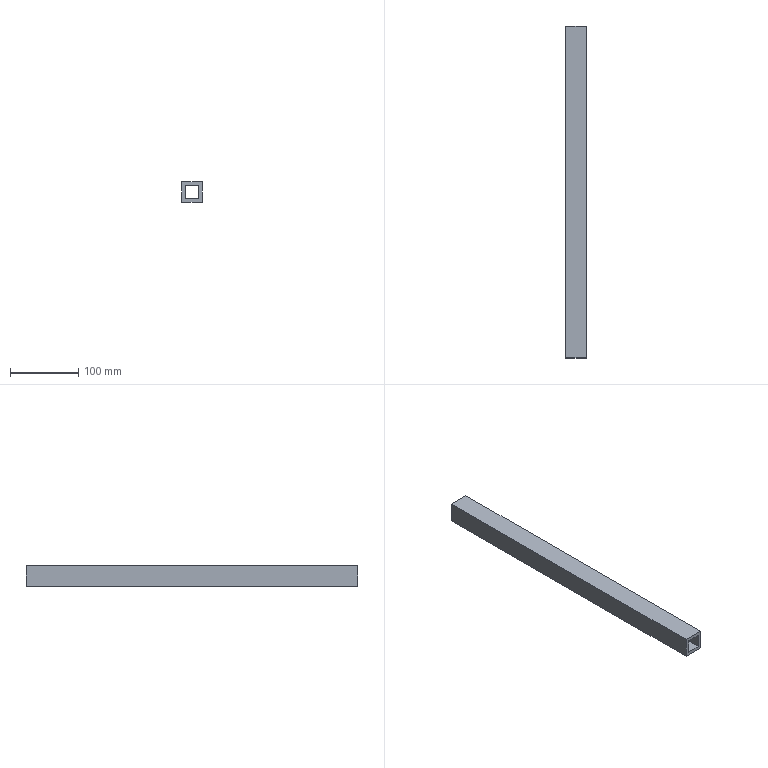Part | NX | features solid 2 | 1 solid | 10 faces | box 30 x 485 x 30 mm | volume 242500 mm3 | plane 10
STEP:
#1=CARTESIAN_POINT('',(175.,-165.,-110.));
#2=VERTEX_POINT('',#1);
#3=CARTESIAN_POINT('',(205.,-165.,-110.));
#4=VERTEX_POINT('',#3);
#5=CARTESIAN_POINT('',(140.,-165.,-110.));
#6=DIRECTION('',(-1.,0.,0.));
#7=VECTOR('',#6,1000.);
#8=LINE('',#5,#7);
#9=EDGE_CURVE('',#2,#4,#8,.F.);
#10=ORIENTED_EDGE('',*,*,#9,.T.);
#11=CARTESIAN_POINT('',(205.,-650.,-110.));
#12=VERTEX_POINT('',#11);
#13=CARTESIAN_POINT('',(205.,20.,-110.));
#14=DIRECTION('',(0.,1.,0.));
#15=VECTOR('',#14,1000.);
#16=LINE('',#13,#15);
#17=EDGE_CURVE('',#12,#4,#16,.T.);
#18=ORIENTED_EDGE('',*,*,#17,.F.);
#19=CARTESIAN_POINT('',(175.,-650.,-110.));
#20=VERTEX_POINT('',#19);
#21=CARTESIAN_POINT('',(-170.,-650.,-110.));
#22=DIRECTION('',(-1.,0.,0.));
#23=VECTOR('',#22,1000.);
#24=LINE('',#21,#23);
#25=EDGE_CURVE('',#20,#12,#24,.F.);
#26=ORIENTED_EDGE('',*,*,#25,.F.);
#27=CARTESIAN_POINT('',(175.,20.,-110.));
#28=DIRECTION('',(0.,1.,0.));
#29=VECTOR('',#28,1000.);
#30=LINE('',#27,#29);
#31=EDGE_CURVE('',#20,#2,#30,.T.);
#32=ORIENTED_EDGE('',*,*,#31,.T.);
#33=EDGE_LOOP('',(#10,#18,#26,#32));
#34=FACE_BOUND('',#33,.T.);
#35=CARTESIAN_POINT('',(205.,20.,-110.));
#36=DIRECTION('',(0.,0.,1.));
#37=DIRECTION('',(0.,1.,0.));
#38=AXIS2_PLACEMENT_3D('',#35,#36,#37);
#39=PLANE('',#38);
#40=ADVANCED_FACE('',(#34),#39,.F.);
#41=CARTESIAN_POINT('',(205.,-165.,-80.));
#42=VERTEX_POINT('',#41);
#43=CARTESIAN_POINT('',(175.,-165.,-80.));
#44=VERTEX_POINT('',#43);
#45=CARTESIAN_POINT('',(140.,-165.,-80.));
#46=DIRECTION('',(-1.,0.,0.));
#47=VECTOR('',#46,1000.);
#48=LINE('',#45,#47);
#49=EDGE_CURVE('',#42,#44,#48,.T.);
#50=ORIENTED_EDGE('',*,*,#49,.T.);
#51=CARTESIAN_POINT('',(175.,-650.,-80.));
#52=VERTEX_POINT('',#51);
#53=CARTESIAN_POINT('',(175.,20.,-80.));
#54=DIRECTION('',(0.,1.,0.));
#55=VECTOR('',#54,1000.);
#56=LINE('',#53,#55);
#57=EDGE_CURVE('',#52,#44,#56,.T.);
#58=ORIENTED_EDGE('',*,*,#57,.F.);
#59=CARTESIAN_POINT('',(205.,-650.,-80.));
#60=VERTEX_POINT('',#59);
#61=CARTESIAN_POINT('',(-170.,-650.,-80.));
#62=DIRECTION('',(-1.,0.,0.));
#63=VECTOR('',#62,1000.);
#64=LINE('',#61,#63);
#65=EDGE_CURVE('',#60,#52,#64,.T.);
#66=ORIENTED_EDGE('',*,*,#65,.F.);
#67=CARTESIAN_POINT('',(205.,20.,-80.));
#68=DIRECTION('',(0.,1.,0.));
#69=VECTOR('',#68,1000.);
#70=LINE('',#67,#69);
#71=EDGE_CURVE('',#60,#42,#70,.T.);
#72=ORIENTED_EDGE('',*,*,#71,.T.);
#73=EDGE_LOOP('',(#50,#58,#66,#72));
#74=FACE_BOUND('',#73,.T.);
#75=CARTESIAN_POINT('',(205.,20.,-80.));
#76=DIRECTION('',(0.,0.,1.));
#77=DIRECTION('',(0.,1.,0.));
#78=AXIS2_PLACEMENT_3D('',#75,#76,#77);
#79=PLANE('',#78);
#80=ADVANCED_FACE('',(#74),#79,.T.);
#81=CARTESIAN_POINT('',(175.,-165.,-50.));
#82=DIRECTION('',(0.,0.,1.));
#83=VECTOR('',#82,1000.);
#84=LINE('',#81,#83);
#85=EDGE_CURVE('',#44,#2,#84,.F.);
#86=ORIENTED_EDGE('',*,*,#85,.T.);
#87=ORIENTED_EDGE('',*,*,#31,.F.);
#88=CARTESIAN_POINT('',(175.,-650.,-45.));
#89=DIRECTION('',(0.,0.,1.));
#90=VECTOR('',#89,1000.);
#91=LINE('',#88,#90);
#92=EDGE_CURVE('',#52,#20,#91,.F.);
#93=ORIENTED_EDGE('',*,*,#92,.F.);
#94=ORIENTED_EDGE('',*,*,#57,.T.);
#95=EDGE_LOOP('',(#86,#87,#93,#94));
#96=FACE_BOUND('',#95,.T.);
#97=CARTESIAN_POINT('',(175.,20.,-80.));
#98=DIRECTION('',(1.,0.,0.));
#99=DIRECTION('',(0.,0.,1.));
#100=AXIS2_PLACEMENT_3D('',#97,#98,#99);
#101=PLANE('',#100);
#102=ADVANCED_FACE('',(#96),#101,.F.);
#103=ORIENTED_EDGE('',*,*,#71,.F.);
#104=CARTESIAN_POINT('',(205.,-650.,-45.));
#105=DIRECTION('',(0.,0.,1.));
#106=VECTOR('',#105,1000.);
#107=LINE('',#104,#106);
#108=EDGE_CURVE('',#60,#12,#107,.F.);
#109=ORIENTED_EDGE('',*,*,#108,.T.);
#110=ORIENTED_EDGE('',*,*,#17,.T.);
#111=CARTESIAN_POINT('',(205.,-165.,-50.));
#112=DIRECTION('',(0.,0.,1.));
#113=VECTOR('',#112,1000.);
#114=LINE('',#111,#113);
#115=EDGE_CURVE('',#42,#4,#114,.F.);
#116=ORIENTED_EDGE('',*,*,#115,.F.);
#117=EDGE_LOOP('',(#103,#109,#110,#116));
#118=FACE_BOUND('',#117,.T.);
#119=CARTESIAN_POINT('',(205.,20.,-80.));
#120=DIRECTION('',(1.,0.,0.));
#121=DIRECTION('',(0.,0.,1.));
#122=AXIS2_PLACEMENT_3D('',#119,#120,#121);
#123=PLANE('',#122);
#124=ADVANCED_FACE('',(#118),#123,.T.);
#125=ORIENTED_EDGE('',*,*,#108,.F.);
#126=ORIENTED_EDGE('',*,*,#65,.T.);
#127=ORIENTED_EDGE('',*,*,#92,.T.);
#128=ORIENTED_EDGE('',*,*,#25,.T.);
#129=EDGE_LOOP('',(#125,#126,#127,#128));
#130=FACE_BOUND('',#129,.T.);
#131=CARTESIAN_POINT('',(200.,-650.,-85.));
#132=VERTEX_POINT('',#131);
#133=CARTESIAN_POINT('',(200.,-650.,-105.));
#134=VERTEX_POINT('',#133);
#135=CARTESIAN_POINT('',(200.,-650.,-45.));
#136=DIRECTION('',(0.,0.,1.));
#137=VECTOR('',#136,1000.);
#138=LINE('',#135,#137);
#139=EDGE_CURVE('',#132,#134,#138,.F.);
#140=ORIENTED_EDGE('',*,*,#139,.T.);
#141=CARTESIAN_POINT('',(180.,-650.,-105.));
#142=VERTEX_POINT('',#141);
#143=CARTESIAN_POINT('',(-170.,-650.,-105.));
#144=DIRECTION('',(-1.,0.,0.));
#145=VECTOR('',#144,1000.);
#146=LINE('',#143,#145);
#147=EDGE_CURVE('',#142,#134,#146,.F.);
#148=ORIENTED_EDGE('',*,*,#147,.F.);
#149=CARTESIAN_POINT('',(180.,-650.,-85.));
#150=VERTEX_POINT('',#149);
#151=CARTESIAN_POINT('',(180.,-650.,-45.));
#152=DIRECTION('',(0.,0.,1.));
#153=VECTOR('',#152,1000.);
#154=LINE('',#151,#153);
#155=EDGE_CURVE('',#150,#142,#154,.F.);
#156=ORIENTED_EDGE('',*,*,#155,.F.);
#157=CARTESIAN_POINT('',(-170.,-650.,-85.));
#158=DIRECTION('',(-1.,0.,0.));
#159=VECTOR('',#158,1000.);
#160=LINE('',#157,#159);
#161=EDGE_CURVE('',#132,#150,#160,.T.);
#162=ORIENTED_EDGE('',*,*,#161,.F.);
#163=EDGE_LOOP('',(#140,#148,#156,#162));
#164=FACE_BOUND('',#163,.T.);
#165=CARTESIAN_POINT('',(-170.,-650.,-45.));
#166=DIRECTION('',(0.,-1.,0.));
#167=DIRECTION('',(-1.,0.,0.));
#168=AXIS2_PLACEMENT_3D('',#165,#166,#167);
#169=PLANE('',#168);
#170=ADVANCED_FACE('',(#130,#164),#169,.T.);
#171=CARTESIAN_POINT('',(180.,-165.,-105.));
#172=VERTEX_POINT('',#171);
#173=CARTESIAN_POINT('',(180.,20.,-105.));
#174=DIRECTION('',(0.,1.,0.));
#175=VECTOR('',#174,1000.);
#176=LINE('',#173,#175);
#177=EDGE_CURVE('',#142,#172,#176,.T.);
#178=ORIENTED_EDGE('',*,*,#177,.F.);
#179=ORIENTED_EDGE('',*,*,#147,.T.);
#180=CARTESIAN_POINT('',(200.,-165.,-105.));
#181=VERTEX_POINT('',#180);
#182=CARTESIAN_POINT('',(200.,20.,-105.));
#183=DIRECTION('',(0.,1.,0.));
#184=VECTOR('',#183,1000.);
#185=LINE('',#182,#184);
#186=EDGE_CURVE('',#134,#181,#185,.T.);
#187=ORIENTED_EDGE('',*,*,#186,.T.);
#188=CARTESIAN_POINT('',(140.,-165.,-105.));
#189=DIRECTION('',(-1.,0.,0.));
#190=VECTOR('',#189,1000.);
#191=LINE('',#188,#190);
#192=EDGE_CURVE('',#172,#181,#191,.F.);
#193=ORIENTED_EDGE('',*,*,#192,.F.);
#194=EDGE_LOOP('',(#178,#179,#187,#193));
#195=FACE_BOUND('',#194,.T.);
#196=CARTESIAN_POINT('',(205.,20.,-105.));
#197=DIRECTION('',(0.,0.,1.));
#198=DIRECTION('',(0.,1.,0.));
#199=AXIS2_PLACEMENT_3D('',#196,#197,#198);
#200=PLANE('',#199);
#201=ADVANCED_FACE('',(#195),#200,.T.);
#202=CARTESIAN_POINT('',(200.,-165.,-85.));
#203=VERTEX_POINT('',#202);
#204=CARTESIAN_POINT('',(200.,20.,-85.));
#205=DIRECTION('',(0.,-1.,0.));
#206=VECTOR('',#205,1000.);
#207=LINE('',#204,#206);
#208=EDGE_CURVE('',#132,#203,#207,.F.);
#209=ORIENTED_EDGE('',*,*,#208,.F.);
#210=ORIENTED_EDGE('',*,*,#161,.T.);
#211=CARTESIAN_POINT('',(180.,-165.,-85.));
#212=VERTEX_POINT('',#211);
#213=CARTESIAN_POINT('',(180.,20.,-85.));
#214=DIRECTION('',(0.,-1.,0.));
#215=VECTOR('',#214,1000.);
#216=LINE('',#213,#215);
#217=EDGE_CURVE('',#150,#212,#216,.F.);
#218=ORIENTED_EDGE('',*,*,#217,.T.);
#219=CARTESIAN_POINT('',(140.,-165.,-85.));
#220=DIRECTION('',(-1.,0.,0.));
#221=VECTOR('',#220,1000.);
#222=LINE('',#219,#221);
#223=EDGE_CURVE('',#203,#212,#222,.T.);
#224=ORIENTED_EDGE('',*,*,#223,.F.);
#225=EDGE_LOOP('',(#209,#210,#218,#224));
#226=FACE_BOUND('',#225,.T.);
#227=CARTESIAN_POINT('',(205.,20.,-85.));
#228=DIRECTION('',(0.,0.,1.));
#229=DIRECTION('',(0.,1.,0.));
#230=AXIS2_PLACEMENT_3D('',#227,#228,#229);
#231=PLANE('',#230);
#232=ADVANCED_FACE('',(#226),#231,.F.);
#233=ORIENTED_EDGE('',*,*,#217,.F.);
#234=ORIENTED_EDGE('',*,*,#155,.T.);
#235=ORIENTED_EDGE('',*,*,#177,.T.);
#236=CARTESIAN_POINT('',(180.,-165.,-50.));
#237=DIRECTION('',(0.,0.,1.));
#238=VECTOR('',#237,1000.);
#239=LINE('',#236,#238);
#240=EDGE_CURVE('',#212,#172,#239,.F.);
#241=ORIENTED_EDGE('',*,*,#240,.F.);
#242=EDGE_LOOP('',(#233,#234,#235,#241));
#243=FACE_BOUND('',#242,.T.);
#244=CARTESIAN_POINT('',(180.,20.,-80.));
#245=DIRECTION('',(1.,0.,0.));
#246=DIRECTION('',(0.,0.,1.));
#247=AXIS2_PLACEMENT_3D('',#244,#245,#246);
#248=PLANE('',#247);
#249=ADVANCED_FACE('',(#243),#248,.T.);
#250=CARTESIAN_POINT('',(200.,-165.,-50.));
#251=DIRECTION('',(0.,0.,1.));
#252=VECTOR('',#251,1000.);
#253=LINE('',#250,#252);
#254=EDGE_CURVE('',#203,#181,#253,.F.);
#255=ORIENTED_EDGE('',*,*,#254,.T.);
#256=ORIENTED_EDGE('',*,*,#186,.F.);
#257=ORIENTED_EDGE('',*,*,#139,.F.);
#258=ORIENTED_EDGE('',*,*,#208,.T.);
#259=EDGE_LOOP('',(#255,#256,#257,#258));
#260=FACE_BOUND('',#259,.T.);
#261=CARTESIAN_POINT('',(200.,20.,-80.));
#262=DIRECTION('',(1.,0.,0.));
#263=DIRECTION('',(0.,0.,1.));
#264=AXIS2_PLACEMENT_3D('',#261,#262,#263);
#265=PLANE('',#264);
#266=ADVANCED_FACE('',(#260),#265,.F.);
#267=ORIENTED_EDGE('',*,*,#192,.T.);
#268=ORIENTED_EDGE('',*,*,#254,.F.);
#269=ORIENTED_EDGE('',*,*,#223,.T.);
#270=ORIENTED_EDGE('',*,*,#240,.T.);
#271=EDGE_LOOP('',(#267,#268,#269,#270));
#272=FACE_BOUND('',#271,.T.);
#273=ORIENTED_EDGE('',*,*,#85,.F.);
#274=ORIENTED_EDGE('',*,*,#49,.F.);
#275=ORIENTED_EDGE('',*,*,#115,.T.);
#276=ORIENTED_EDGE('',*,*,#9,.F.);
#277=EDGE_LOOP('',(#273,#274,#275,#276));
#278=FACE_BOUND('',#277,.T.);
#279=CARTESIAN_POINT('',(140.,-165.,-50.));
#280=DIRECTION('',(0.,-1.,0.));
#281=DIRECTION('',(0.,0.,-1.));
#282=AXIS2_PLACEMENT_3D('',#279,#280,#281);
#283=PLANE('',#282);
#284=ADVANCED_FACE('',(#272,#278),#283,.F.);
#285=CLOSED_SHELL('',(#40,#80,#102,#124,#170,#201,#232,#249,#266,#284));
#286=MANIFOLD_SOLID_BREP('',#285);
#287=(LENGTH_UNIT()NAMED_UNIT(*)SI_UNIT(.MILLI.,.METRE.));
#288=UNCERTAINTY_MEASURE_WITH_UNIT(LENGTH_MEASURE(0.00001),#287,'','');
#289=(NAMED_UNIT(*)PLANE_ANGLE_UNIT()SI_UNIT($,.RADIAN.));
#290=(NAMED_UNIT(*)SI_UNIT($,.STERADIAN.)SOLID_ANGLE_UNIT());
#291=(GEOMETRIC_REPRESENTATION_CONTEXT(3)GLOBAL_UNCERTAINTY_ASSIGNED_CONTEXT((#288))GLOBAL_UNIT_ASSIGNED_CONTEXT((#287,#289,#290))REPRESENTATION_CONTEXT('',''));
#292=ADVANCED_BREP_SHAPE_REPRESENTATION('',(#286),#291);